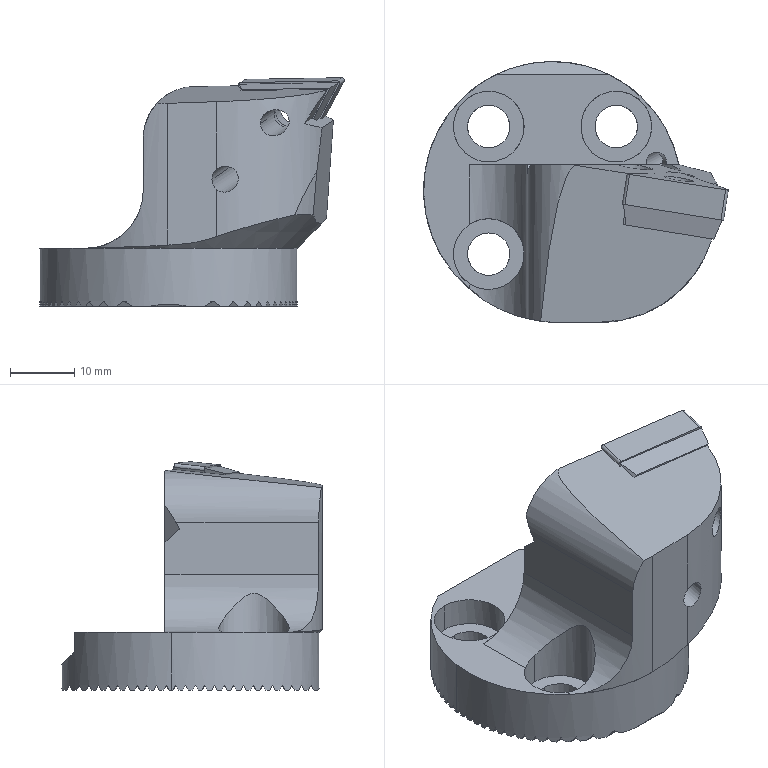NC program | Mastercam | posted with a generic post
Lines 1 to 242 of 11065:
%
:0001()
(MATERIAL - ALUMINUM MM - 2024)
(T18|8 FEM |H18)
(T2|5 CHM |H2)
(T13|3.3 DR |H13)
(T17|2.9 DR |H17)
(T4|12 FEMR |H4|XY STOCK TO LEAVE - .1|Z STOCK TO LEAVE - 0.)
(T5|6 FEMR |H5|XY STOCK TO LEAVE - .1|Z STOCK TO LEAVE - .05)
(T6|4 FEMR |H6|D6|WEAR COMP|TOOL DIA. - 4.|XY STOCK TO LEAVE - .07|Z STOCK TO LEAVE - .05)
(T9|12 FEMF |H9|D9|WEAR COMP|TOOL DIA. - 12.)
(T10|30 INC |H10|D10|WEAR COMP|TOOL DIA. - 30.)
(T12|6 CHM |H12)
(T3|6 DR |H3)
(T11|4.5 FEM |H11)
(T14|M4 XXXXXX |H14|D14|WEAR COMP|TOOL DIA. - 3.15)
(T16|M4 X 0.7 RH |H16)
(T1|1.6 DR |H1)
(T7|4 FEMF |H7|D7|WEAR COMP|TOOL DIA. - 4.)
(T15|2.5 BM |H15)
N100 G21
N102 G0 G17 G40 G80 G90 G94 G98
N104 G0 G28 G91 Z0.
N106 G0 G28 X0. Y0.
(8 FEM |TOOL - 18|DIA. OFF. - 18|LEN. - 18|TOOL DIA. - 8.)
N108 T18 M6
N110 G0 G54 G90 X-21.518 Y-5.5 C90. B-22.5 S3500 M3
N112 G43 H18 Z92.075
N114 Z43.075
N116 G1 Z41.783 F2000.
N118 X-15.518 F1500.
N120 X-11.474
N122 X-5.474
N124 G0 Z50.
N126 X-21.518
N128 Z42.783
N130 G1 Z41.491 F2000.
N132 X-15.518 F1500.
N134 X-11.474
N136 X-5.474
N138 G0 Z50.
N140 X-21.518
N142 Z42.491
N144 G1 Z41.2 F2000.
N146 X-15.518 F1500.
N148 X-11.474
N150 X-5.474
N152 G0 Z50.
N154 X-21.518
N156 Z42.2
N158 G1 Z40.908 F2000.
N160 X-15.518 F1500.
N162 X-11.474
N164 X-5.474
N166 G0 Z50.
N168 X-21.518
N170 Z41.908
N172 G1 Z40.616 F2000.
N174 X-15.518 F1500.
N176 X-11.474
N178 X-5.474
N180 G0 Z50.
N182 X-21.518
N184 Z41.616
N186 G1 Z40.325 F2000.
N188 X-15.518 F1500.
N190 X-11.474
N192 X-5.474
N194 G0 Z50.
N196 X-21.518
N198 Z41.325
N200 G1 Z40.033 F2000.
N202 X-15.518 F1500.
N204 X-11.474
N206 X-5.474
N208 G0 Z50.
N210 X-21.518
N212 Z41.033
N214 G1 Z39.741 F2000.
N216 X-15.518 F1500.
N218 X-11.474
N220 X-5.474
N222 G0 Z50.
N224 X-21.518
N226 Z40.741
N228 G1 Z39.45 F2000.
N230 X-15.518 F1500.
N232 X-11.474
N234 X-5.474
N236 G0 Z50.
N238 X-21.518
N240 Z40.45
N242 G1 Z39.158 F2000.
N244 X-15.518 F1500.
N246 X-11.474
N248 X-5.474
N250 G0 Z50.
N252 X-21.518
N254 Z40.158
N256 G1 Z38.866 F2000.
N258 X-15.518 F1500.
N260 X-11.474
N262 X-5.474
N264 G0 Z50.
N266 X-21.518
N268 Z39.866
N270 G1 Z38.575 F2000.
N272 X-15.518 F1500.
N274 X-11.474
N276 X-5.474
N278 G0 Z50.
N280 X-21.518
N282 Z39.575
N284 G1 Z38.283 F2000.
N286 X-15.518 F1500.
N288 X-11.474
N290 X-5.474
N292 G0 Z50.
N294 X-21.518
N296 Z39.283
N298 G1 Z37.991 F2000.
N300 X-15.518 F1500.
N302 X-11.474
N304 X-5.474
N306 G0 Z50.
N308 X-21.518
N310 Z38.991
N312 G1 Z37.7 F2000.
N314 X-15.518 F1500.
N316 X-11.474
N318 X-5.474
N320 G0 Z50.
N322 X-21.518
N324 Z38.7
N326 G1 Z37.408 F2000.
N328 X-15.518 F1500.
N330 X-11.474
N332 X-5.474
N334 G0 Z50.
N336 X-21.518
N338 Z38.408
N340 G1 Z37.116 F2000.
N342 X-15.518 F1500.
N344 X-11.474
N346 X-5.474
N348 G0 Z50.
N350 X-21.518
N352 Z38.116
N354 G1 Z36.825 F2000.
N356 X-15.518 F1500.
N358 X-11.474
N360 X-5.474
N362 G0 Z50.
N364 X-21.518
N366 Z37.825
N368 G1 Z36.533 F2000.
N370 X-15.518 F1500.
N372 X-11.474
N374 X-5.474
N376 G0 Z50.
N378 X-21.518
N380 Z37.533
N382 G1 Z36.241 F2000.
N384 X-15.518 F1500.
N386 X-11.474
N388 X-5.474
N390 G0 Z50.
N392 X-21.518
N394 Z37.241
N396 G1 Z35.95 F2000.
N398 X-15.518 F1500.
N400 X-11.474
N402 X-5.474
N404 G0 Z50.
N406 X-21.518
N408 Z36.95
N410 G1 Z35.658 F2000.
N412 X-15.518 F1500.
N414 X-11.474
N416 X-5.474
N418 G0 Z50.
N420 X-21.518
N422 Z36.658
N424 G1 Z35.366 F2000.
N426 X-15.518 F1500.
N428 X-11.474
N430 X-5.474
N432 G0 Z50.
N434 X-21.518
N436 Z36.366
N438 G1 Z35.075 F2000.
N440 X-15.518 F1500.
N442 X-11.474
N444 X-5.474
N446 G0 Z92.075
N448 M5
N450 G0 G28 G91 Z0.
N452 G28 C0. B0.
N454 M01
N456 G0 G17 G40 G80 G90 G94 G98
N458 G0 G28 G91 Z0.
(5 CHM |TOOL - 2|DIA. OFF. - 2|LEN. - 2|TOOL DIA. - 5.)
N460 T2 M6
N462 G0 G54 G90 X-11.474 Y-4.5 C90. B-22.5 S2000 M3
N464 G43 H2 Z85.075
N466 G81 G98 Z34.075 R36.075 F100.
N468 G80
N470 C64. B-90.
N472 X6. Y3.
N474 Z69.954
N476 G81 G98 Z18.454 R20.954 F100.
N478 G80
N480 M5
N482 G0 G28 G91 Z0.
N484 G28 C0. B0.
N486 M01
N488 G0 G17 G40 G80 G90 G94 G98
N490 G0 G28 G91 Z0.
(3.3 DR |TOOL - 13|DIA. OFF. - 13|LEN. - 13|TOOL DIA. - 3.3)
N492 T13 M6
N494 G0 G54 G90 X6. Y3. C64. B-90. S3000 M3
N496 G43 H13 Z69.954
N498 G83 G98 Z-.046 R20.954 Q1. F60.
N500 G80
N502 M5
N504 G0 G28 G91 Z0.
N506 G28 C0. B0.
N508 M01
N510 G0 G17 G40 G80 G90 G94 G98
N512 G0 G28 G91 Z0.
(2.9 DR |TOOL - 17|DIA. OFF. - 17|LEN. - 17|TOOL DIA. - 2.9)
N514 T17 M6
N516 G0 G54 G90 X-11.474 Y-4.5 C90. B-22.5 S3000 M3
N518 G43 H17 Z85.075
N520 G83 G98 Z10.575 R36.075 Q2. F60.
N522 G80
N524 M5
N526 G0 G28 G91 Z0.
N528 G28 C0. B0.
N530 M01
N532 G0 G17 G40 G80 G90 G94 G98
N534 G0 G28 G91 Z0.